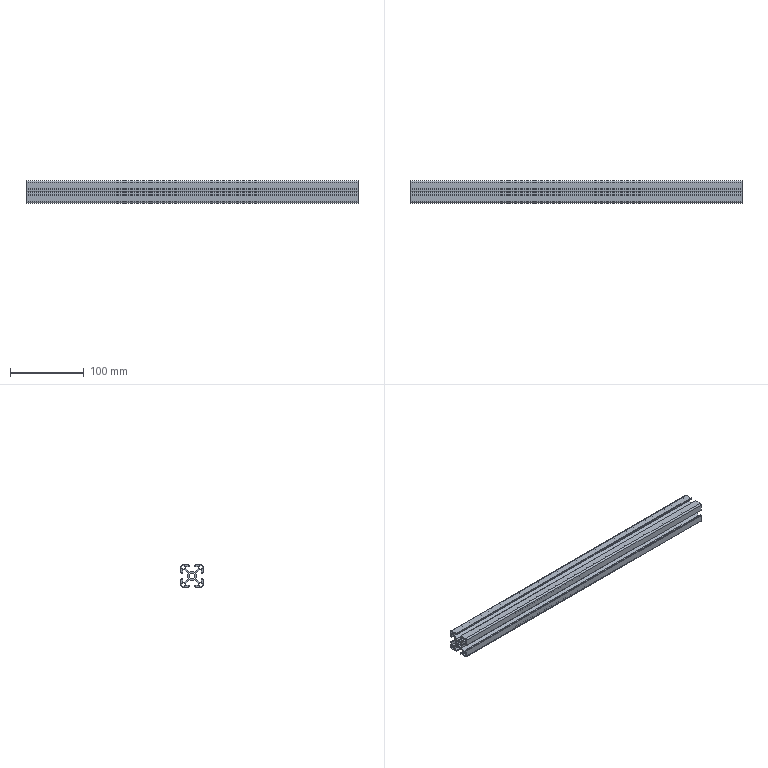Part | STEP file | PERFIL_30X30_450 | 1 solid | 126 faces | box 450 x 30 x 30 mm | volume 139687 mm3 | plane 98 | cylinder 27 | spline 1 | commonest cylinder face diameters 2 x16 4 x4 11 x4 8 x3